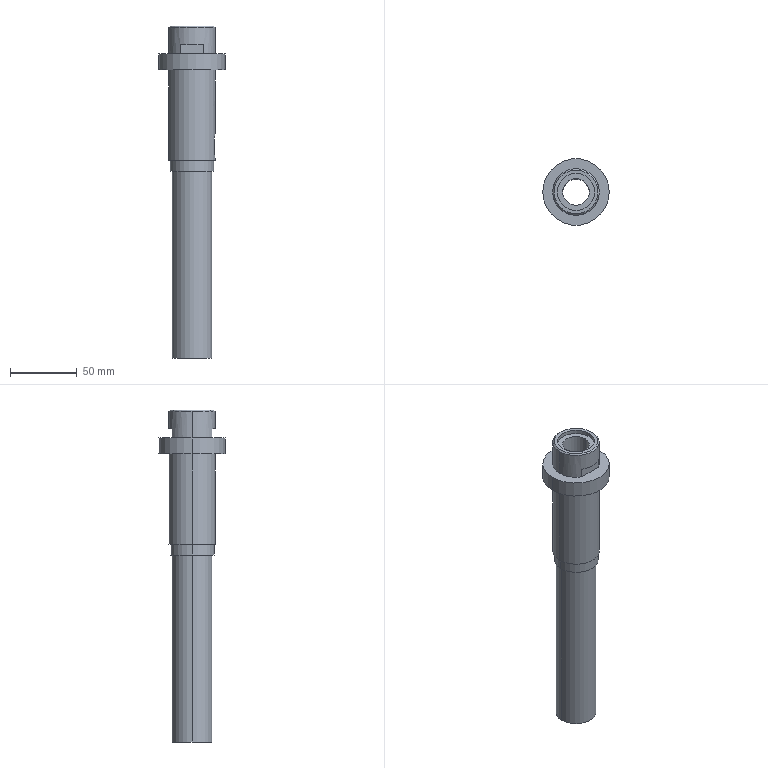Part | STEP file | Double-tube discharge pipe SGN-2-06 | 1 solid | 33 faces | box 50 x 50 x 249.5 mm | volume 134723 mm3 | cylinder 17 | plane 14 | cone 2 | commonest cylinder face diameters 35 x4 10 x3 20 x2 28 x2 30 x2 33 x2